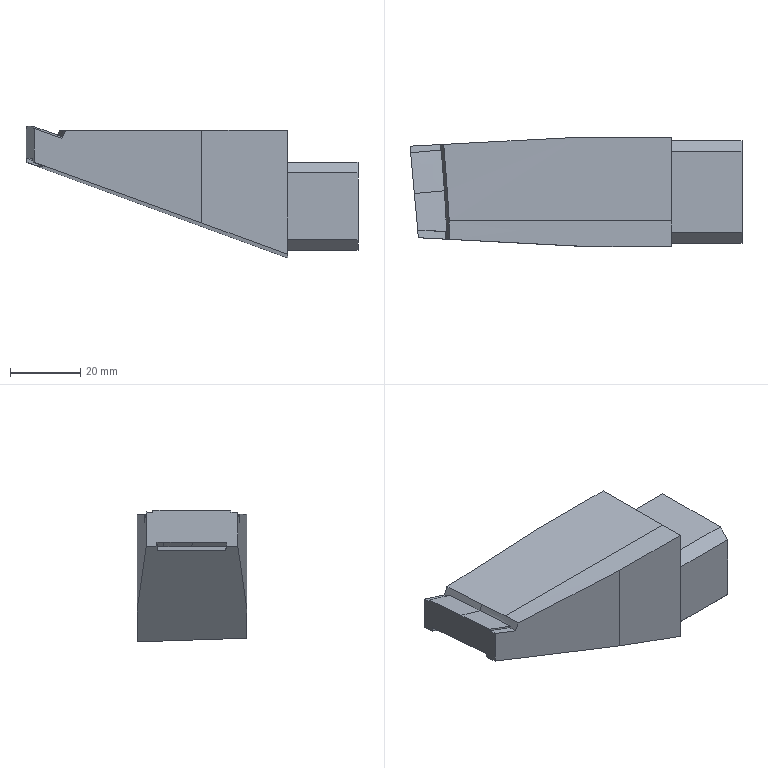Part | STEP file | P011002S002-003 | 1 solid | 67 faces | box 94.285 x 31 x 37.408 mm | volume 61974 mm3 | plane 35 | other 13 | spline 9 | cone 7 | cylinder 3 | commonest cylinder face diameters 6.8 x1 7.973 x1 8 x1